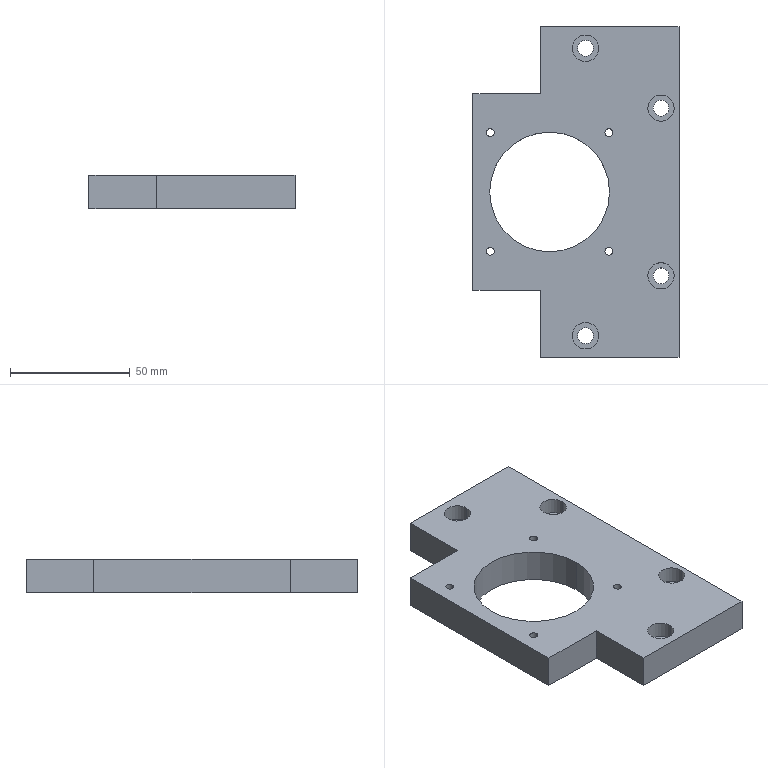Part | STEP file | PN_0041 motor spacer block | 1 solid | 40 faces | box 86 x 138 x 14 mm | volume 112662 mm3 | cylinder 26 | plane 14 | commonest cylinder face diameters 3.3 x8 6.6 x8 11 x8 50 x2